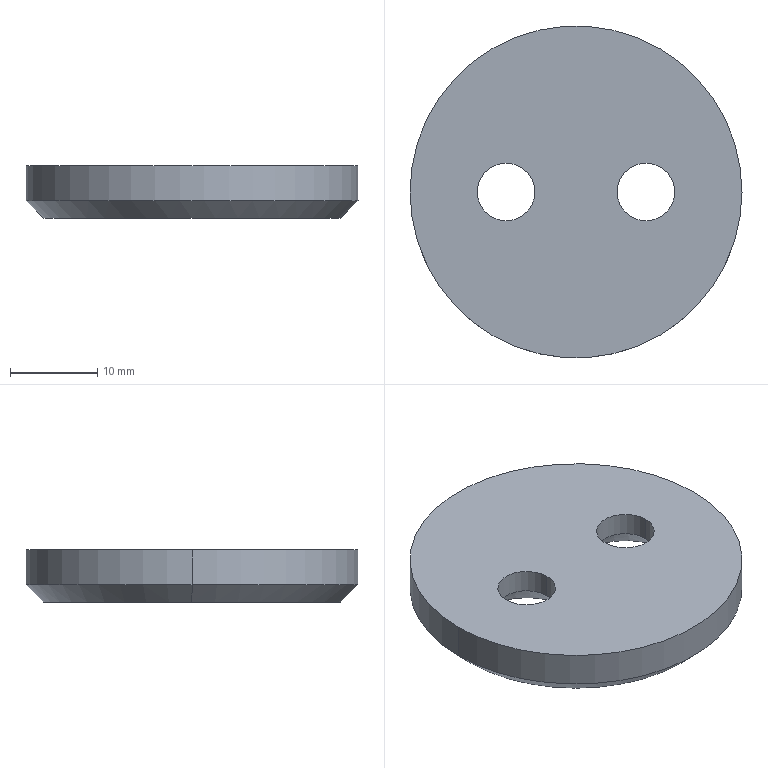Part | SolidWorks | features BaseBody 1 | 1 solid | 14 faces | box 38 x 38 x 6 mm | volume 5863 mm3 | cone 6 | cylinder 6 | plane 2 | commonest cylinder face diameters 6.6 x4 38 x2
STEP:
#1=CARTESIAN_POINT('',(11.3,0.,0.3));
#2=VERTEX_POINT('',#1);
#3=CARTESIAN_POINT('',(4.7,0.,0.3));
#4=VERTEX_POINT('',#3);
#5=CARTESIAN_POINT('',(8.,0.,0.3));
#6=DIRECTION('',(0.,0.,-1.));
#7=DIRECTION('',(-1.,0.,0.));
#8=AXIS2_PLACEMENT_3D('',#5,#6,#7);
#9=CIRCLE('',#8,3.3);
#10=EDGE_CURVE('',#2,#4,#9,.T.);
#11=ORIENTED_EDGE('',*,*,#10,.F.);
#12=CARTESIAN_POINT('',(14.6,0.,-3.));
#13=VERTEX_POINT('',#12);
#14=CARTESIAN_POINT('',(14.6,0.,-3.));
#15=DIRECTION('',(0.7071,0.,-0.7071));
#16=VECTOR('',#15,1000.);
#17=LINE('',#14,#16);
#18=EDGE_CURVE('',#2,#13,#17,.T.);
#19=ORIENTED_EDGE('',*,*,#18,.T.);
#20=CARTESIAN_POINT('',(1.4,0.,-3.));
#21=VERTEX_POINT('',#20);
#22=CARTESIAN_POINT('',(8.,0.,-3.));
#23=DIRECTION('',(0.,0.,-1.));
#24=DIRECTION('',(-1.,0.,0.));
#25=AXIS2_PLACEMENT_3D('',#22,#23,#24);
#26=CIRCLE('',#25,6.6);
#27=EDGE_CURVE('',#13,#21,#26,.T.);
#28=ORIENTED_EDGE('',*,*,#27,.T.);
#29=CARTESIAN_POINT('',(1.4,0.,-3.));
#30=DIRECTION('',(-0.7071,0.,-0.7071));
#31=VECTOR('',#30,1000.);
#32=LINE('',#29,#31);
#33=EDGE_CURVE('',#4,#21,#32,.T.);
#34=ORIENTED_EDGE('',*,*,#33,.F.);
#35=EDGE_LOOP('',(#11,#19,#28,#34));
#36=FACE_OUTER_BOUND('',#35,.T.);
#37=CARTESIAN_POINT('',(8.,0.,-3.));
#38=DIRECTION('',(0.,0.,-1.));
#39=DIRECTION('',(-1.,0.,0.));
#40=AXIS2_PLACEMENT_3D('',#37,#38,#39);
#41=CONICAL_SURFACE('',#40,6.6,0.7854);
#42=ADVANCED_FACE('',(#36),#41,.F.);
#43=CARTESIAN_POINT('',(11.3,0.,3.));
#44=VERTEX_POINT('',#43);
#45=CARTESIAN_POINT('',(4.7,0.,3.));
#46=VERTEX_POINT('',#45);
#47=CARTESIAN_POINT('',(8.,0.,3.));
#48=DIRECTION('',(0.,0.,-1.));
#49=DIRECTION('',(-1.,0.,0.));
#50=AXIS2_PLACEMENT_3D('',#47,#48,#49);
#51=CIRCLE('',#50,3.3);
#52=EDGE_CURVE('',#44,#46,#51,.T.);
#53=ORIENTED_EDGE('',*,*,#52,.F.);
#54=CARTESIAN_POINT('',(11.3,0.,-3.));
#55=DIRECTION('',(0.,0.,-1.));
#56=VECTOR('',#55,1000.);
#57=LINE('',#54,#56);
#58=EDGE_CURVE('',#44,#2,#57,.T.);
#59=ORIENTED_EDGE('',*,*,#58,.T.);
#60=ORIENTED_EDGE('',*,*,#10,.T.);
#61=CARTESIAN_POINT('',(4.7,0.,-3.));
#62=DIRECTION('',(0.,0.,-1.));
#63=VECTOR('',#62,1000.);
#64=LINE('',#61,#63);
#65=EDGE_CURVE('',#46,#4,#64,.T.);
#66=ORIENTED_EDGE('',*,*,#65,.F.);
#67=EDGE_LOOP('',(#53,#59,#60,#66));
#68=FACE_OUTER_BOUND('',#67,.T.);
#69=CARTESIAN_POINT('',(8.,0.,-3.));
#70=DIRECTION('',(0.,0.,-1.));
#71=DIRECTION('',(-1.,0.,0.));
#72=AXIS2_PLACEMENT_3D('',#69,#70,#71);
#73=CYLINDRICAL_SURFACE('',#72,3.3);
#74=ADVANCED_FACE('',(#68),#73,.F.);
#75=CARTESIAN_POINT('',(-4.7,0.,0.3));
#76=VERTEX_POINT('',#75);
#77=CARTESIAN_POINT('',(-11.3,0.,0.3));
#78=VERTEX_POINT('',#77);
#79=CARTESIAN_POINT('',(-8.,0.,0.3));
#80=DIRECTION('',(0.,0.,-1.));
#81=DIRECTION('',(-1.,0.,0.));
#82=AXIS2_PLACEMENT_3D('',#79,#80,#81);
#83=CIRCLE('',#82,3.3);
#84=EDGE_CURVE('',#76,#78,#83,.T.);
#85=ORIENTED_EDGE('',*,*,#84,.F.);
#86=CARTESIAN_POINT('',(-1.4,0.,-3.));
#87=VERTEX_POINT('',#86);
#88=CARTESIAN_POINT('',(-1.4,0.,-3.));
#89=DIRECTION('',(0.7071,0.,-0.7071));
#90=VECTOR('',#89,1000.);
#91=LINE('',#88,#90);
#92=EDGE_CURVE('',#76,#87,#91,.T.);
#93=ORIENTED_EDGE('',*,*,#92,.T.);
#94=CARTESIAN_POINT('',(-14.6,0.,-3.));
#95=VERTEX_POINT('',#94);
#96=CARTESIAN_POINT('',(-8.,0.,-3.));
#97=DIRECTION('',(0.,0.,-1.));
#98=DIRECTION('',(-1.,0.,0.));
#99=AXIS2_PLACEMENT_3D('',#96,#97,#98);
#100=CIRCLE('',#99,6.6);
#101=EDGE_CURVE('',#87,#95,#100,.T.);
#102=ORIENTED_EDGE('',*,*,#101,.T.);
#103=CARTESIAN_POINT('',(-14.6,0.,-3.));
#104=DIRECTION('',(-0.7071,0.,-0.7071));
#105=VECTOR('',#104,1000.);
#106=LINE('',#103,#105);
#107=EDGE_CURVE('',#78,#95,#106,.T.);
#108=ORIENTED_EDGE('',*,*,#107,.F.);
#109=EDGE_LOOP('',(#85,#93,#102,#108));
#110=FACE_OUTER_BOUND('',#109,.T.);
#111=CARTESIAN_POINT('',(-8.,0.,-3.));
#112=DIRECTION('',(0.,0.,-1.));
#113=DIRECTION('',(-1.,0.,0.));
#114=AXIS2_PLACEMENT_3D('',#111,#112,#113);
#115=CONICAL_SURFACE('',#114,6.6,0.7854);
#116=ADVANCED_FACE('',(#110),#115,.F.);
#117=CARTESIAN_POINT('',(-4.7,0.,3.));
#118=VERTEX_POINT('',#117);
#119=CARTESIAN_POINT('',(-11.3,0.,3.));
#120=VERTEX_POINT('',#119);
#121=CARTESIAN_POINT('',(-8.,0.,3.));
#122=DIRECTION('',(0.,0.,-1.));
#123=DIRECTION('',(-1.,0.,0.));
#124=AXIS2_PLACEMENT_3D('',#121,#122,#123);
#125=CIRCLE('',#124,3.3);
#126=EDGE_CURVE('',#118,#120,#125,.T.);
#127=ORIENTED_EDGE('',*,*,#126,.F.);
#128=CARTESIAN_POINT('',(-4.7,0.,-3.));
#129=DIRECTION('',(0.,0.,-1.));
#130=VECTOR('',#129,1000.);
#131=LINE('',#128,#130);
#132=EDGE_CURVE('',#118,#76,#131,.T.);
#133=ORIENTED_EDGE('',*,*,#132,.T.);
#134=ORIENTED_EDGE('',*,*,#84,.T.);
#135=CARTESIAN_POINT('',(-11.3,0.,-3.));
#136=DIRECTION('',(0.,0.,-1.));
#137=VECTOR('',#136,1000.);
#138=LINE('',#135,#137);
#139=EDGE_CURVE('',#120,#78,#138,.T.);
#140=ORIENTED_EDGE('',*,*,#139,.F.);
#141=EDGE_LOOP('',(#127,#133,#134,#140));
#142=FACE_OUTER_BOUND('',#141,.T.);
#143=CARTESIAN_POINT('',(-8.,0.,-3.));
#144=DIRECTION('',(0.,0.,-1.));
#145=DIRECTION('',(-1.,0.,0.));
#146=AXIS2_PLACEMENT_3D('',#143,#144,#145);
#147=CYLINDRICAL_SURFACE('',#146,3.3);
#148=ADVANCED_FACE('',(#142),#147,.F.);
#149=CARTESIAN_POINT('',(-17.,0.,-3.));
#150=VERTEX_POINT('',#149);
#151=CARTESIAN_POINT('',(17.,0.,-3.));
#152=VERTEX_POINT('',#151);
#153=CARTESIAN_POINT('',(0.,0.,-3.));
#154=DIRECTION('',(0.,0.,-1.));
#155=DIRECTION('',(1.,0.,0.));
#156=AXIS2_PLACEMENT_3D('',#153,#154,#155);
#157=CIRCLE('',#156,17.);
#158=EDGE_CURVE('',#150,#152,#157,.T.);
#159=ORIENTED_EDGE('',*,*,#158,.F.);
#160=CARTESIAN_POINT('',(-19.,0.,-1.));
#161=VERTEX_POINT('',#160);
#162=CARTESIAN_POINT('',(-19.,0.,-1.));
#163=DIRECTION('',(-0.7071,0.,0.7071));
#164=VECTOR('',#163,1000.);
#165=LINE('',#162,#164);
#166=EDGE_CURVE('',#150,#161,#165,.T.);
#167=ORIENTED_EDGE('',*,*,#166,.T.);
#168=CARTESIAN_POINT('',(19.,0.,-1.));
#169=VERTEX_POINT('',#168);
#170=CARTESIAN_POINT('',(0.,0.,-1.));
#171=DIRECTION('',(0.,0.,1.));
#172=DIRECTION('',(1.,0.,0.));
#173=AXIS2_PLACEMENT_3D('',#170,#171,#172);
#174=CIRCLE('',#173,19.);
#175=EDGE_CURVE('',#169,#161,#174,.T.);
#176=ORIENTED_EDGE('',*,*,#175,.F.);
#177=CARTESIAN_POINT('',(19.,0.,-1.));
#178=DIRECTION('',(0.7071,0.,0.7071));
#179=VECTOR('',#178,1000.);
#180=LINE('',#177,#179);
#181=EDGE_CURVE('',#152,#169,#180,.T.);
#182=ORIENTED_EDGE('',*,*,#181,.F.);
#183=EDGE_LOOP('',(#159,#167,#176,#182));
#184=FACE_OUTER_BOUND('',#183,.T.);
#185=CARTESIAN_POINT('',(0.,0.,-1.));
#186=DIRECTION('',(0.,0.,1.));
#187=DIRECTION('',(1.,0.,0.));
#188=AXIS2_PLACEMENT_3D('',#185,#186,#187);
#189=CONICAL_SURFACE('',#188,19.,0.7854);
#190=ADVANCED_FACE('',(#184),#189,.T.);
#191=CARTESIAN_POINT('',(19.,0.,3.));
#192=VERTEX_POINT('',#191);
#193=CARTESIAN_POINT('',(-19.,0.,3.));
#194=VERTEX_POINT('',#193);
#195=CARTESIAN_POINT('',(0.,0.,3.));
#196=DIRECTION('',(0.,0.,1.));
#197=DIRECTION('',(1.,0.,0.));
#198=AXIS2_PLACEMENT_3D('',#195,#196,#197);
#199=CIRCLE('',#198,19.);
#200=EDGE_CURVE('',#192,#194,#199,.T.);
#201=ORIENTED_EDGE('',*,*,#200,.F.);
#202=CARTESIAN_POINT('',(19.,0.,3.));
#203=DIRECTION('',(0.,0.,-1.));
#204=VECTOR('',#203,1000.);
#205=LINE('',#202,#204);
#206=EDGE_CURVE('',#192,#169,#205,.T.);
#207=ORIENTED_EDGE('',*,*,#206,.T.);
#208=ORIENTED_EDGE('',*,*,#175,.T.);
#209=CARTESIAN_POINT('',(-19.,0.,3.));
#210=DIRECTION('',(0.,0.,-1.));
#211=VECTOR('',#210,1000.);
#212=LINE('',#209,#211);
#213=EDGE_CURVE('',#194,#161,#212,.T.);
#214=ORIENTED_EDGE('',*,*,#213,.F.);
#215=EDGE_LOOP('',(#201,#207,#208,#214));
#216=FACE_OUTER_BOUND('',#215,.T.);
#217=CARTESIAN_POINT('',(0.,0.,3.));
#218=DIRECTION('',(0.,0.,-1.));
#219=DIRECTION('',(-1.,0.,0.));
#220=AXIS2_PLACEMENT_3D('',#217,#218,#219);
#221=CYLINDRICAL_SURFACE('',#220,19.);
#222=ADVANCED_FACE('',(#216),#221,.T.);
#223=CARTESIAN_POINT('',(-8.,0.,-3.));
#224=DIRECTION('',(0.,0.,-1.));
#225=DIRECTION('',(-1.,0.,0.));
#226=AXIS2_PLACEMENT_3D('',#223,#224,#225);
#227=CIRCLE('',#226,6.6);
#228=EDGE_CURVE('',#95,#87,#227,.T.);
#229=ORIENTED_EDGE('',*,*,#228,.F.);
#230=ORIENTED_EDGE('',*,*,#101,.F.);
#231=EDGE_LOOP('',(#229,#230));
#232=FACE_BOUND('',#231,.T.);
#233=CARTESIAN_POINT('',(8.,0.,-3.));
#234=DIRECTION('',(0.,0.,-1.));
#235=DIRECTION('',(-1.,0.,0.));
#236=AXIS2_PLACEMENT_3D('',#233,#234,#235);
#237=CIRCLE('',#236,6.6);
#238=EDGE_CURVE('',#21,#13,#237,.T.);
#239=ORIENTED_EDGE('',*,*,#238,.F.);
#240=ORIENTED_EDGE('',*,*,#27,.F.);
#241=EDGE_LOOP('',(#239,#240));
#242=FACE_BOUND('',#241,.T.);
#243=CARTESIAN_POINT('',(0.,0.,-3.));
#244=DIRECTION('',(0.,0.,-1.));
#245=DIRECTION('',(1.,0.,0.));
#246=AXIS2_PLACEMENT_3D('',#243,#244,#245);
#247=CIRCLE('',#246,17.);
#248=EDGE_CURVE('',#152,#150,#247,.T.);
#249=ORIENTED_EDGE('',*,*,#248,.T.);
#250=ORIENTED_EDGE('',*,*,#158,.T.);
#251=EDGE_LOOP('',(#249,#250));
#252=FACE_OUTER_BOUND('',#251,.T.);
#253=CARTESIAN_POINT('',(0.,0.,-3.));
#254=DIRECTION('',(0.,0.,1.));
#255=DIRECTION('',(0.,-1.,0.));
#256=AXIS2_PLACEMENT_3D('',#253,#254,#255);
#257=PLANE('',#256);
#258=ADVANCED_FACE('',(#232,#242,#252),#257,.F.);
#259=CARTESIAN_POINT('',(-8.,0.,3.));
#260=DIRECTION('',(0.,0.,-1.));
#261=DIRECTION('',(-1.,0.,0.));
#262=AXIS2_PLACEMENT_3D('',#259,#260,#261);
#263=CIRCLE('',#262,3.3);
#264=EDGE_CURVE('',#120,#118,#263,.T.);
#265=ORIENTED_EDGE('',*,*,#264,.T.);
#266=ORIENTED_EDGE('',*,*,#126,.T.);
#267=EDGE_LOOP('',(#265,#266));
#268=FACE_BOUND('',#267,.T.);
#269=CARTESIAN_POINT('',(8.,0.,3.));
#270=DIRECTION('',(0.,0.,-1.));
#271=DIRECTION('',(-1.,0.,0.));
#272=AXIS2_PLACEMENT_3D('',#269,#270,#271);
#273=CIRCLE('',#272,3.3);
#274=EDGE_CURVE('',#46,#44,#273,.T.);
#275=ORIENTED_EDGE('',*,*,#274,.T.);
#276=ORIENTED_EDGE('',*,*,#52,.T.);
#277=EDGE_LOOP('',(#275,#276));
#278=FACE_BOUND('',#277,.T.);
#279=CARTESIAN_POINT('',(0.,0.,3.));
#280=DIRECTION('',(0.,0.,1.));
#281=DIRECTION('',(1.,0.,0.));
#282=AXIS2_PLACEMENT_3D('',#279,#280,#281);
#283=CIRCLE('',#282,19.);
#284=EDGE_CURVE('',#194,#192,#283,.T.);
#285=ORIENTED_EDGE('',*,*,#284,.T.);
#286=ORIENTED_EDGE('',*,*,#200,.T.);
#287=EDGE_LOOP('',(#285,#286));
#288=FACE_OUTER_BOUND('',#287,.T.);
#289=CARTESIAN_POINT('',(0.,0.,3.));
#290=DIRECTION('',(0.,0.,1.));
#291=DIRECTION('',(0.,-1.,0.));
#292=AXIS2_PLACEMENT_3D('',#289,#290,#291);
#293=PLANE('',#292);
#294=ADVANCED_FACE('',(#268,#278,#288),#293,.T.);
#295=ORIENTED_EDGE('',*,*,#206,.F.);
#296=ORIENTED_EDGE('',*,*,#284,.F.);
#297=ORIENTED_EDGE('',*,*,#213,.T.);
#298=CARTESIAN_POINT('',(0.,0.,-1.));
#299=DIRECTION('',(0.,0.,1.));
#300=DIRECTION('',(1.,0.,0.));
#301=AXIS2_PLACEMENT_3D('',#298,#299,#300);
#302=CIRCLE('',#301,19.);
#303=EDGE_CURVE('',#161,#169,#302,.T.);
#304=ORIENTED_EDGE('',*,*,#303,.T.);
#305=EDGE_LOOP('',(#295,#296,#297,#304));
#306=FACE_OUTER_BOUND('',#305,.T.);
#307=CARTESIAN_POINT('',(0.,0.,3.));
#308=DIRECTION('',(0.,0.,-1.));
#309=DIRECTION('',(-1.,0.,0.));
#310=AXIS2_PLACEMENT_3D('',#307,#308,#309);
#311=CYLINDRICAL_SURFACE('',#310,19.);
#312=ADVANCED_FACE('',(#306),#311,.T.);
#313=ORIENTED_EDGE('',*,*,#166,.F.);
#314=ORIENTED_EDGE('',*,*,#248,.F.);
#315=ORIENTED_EDGE('',*,*,#181,.T.);
#316=ORIENTED_EDGE('',*,*,#303,.F.);
#317=EDGE_LOOP('',(#313,#314,#315,#316));
#318=FACE_OUTER_BOUND('',#317,.T.);
#319=CARTESIAN_POINT('',(0.,0.,-1.));
#320=DIRECTION('',(0.,0.,1.));
#321=DIRECTION('',(1.,0.,0.));
#322=AXIS2_PLACEMENT_3D('',#319,#320,#321);
#323=CONICAL_SURFACE('',#322,19.,0.7854);
#324=ADVANCED_FACE('',(#318),#323,.T.);
#325=ORIENTED_EDGE('',*,*,#132,.F.);
#326=ORIENTED_EDGE('',*,*,#264,.F.);
#327=ORIENTED_EDGE('',*,*,#139,.T.);
#328=CARTESIAN_POINT('',(-8.,0.,0.3));
#329=DIRECTION('',(0.,0.,-1.));
#330=DIRECTION('',(-1.,0.,0.));
#331=AXIS2_PLACEMENT_3D('',#328,#329,#330);
#332=CIRCLE('',#331,3.3);
#333=EDGE_CURVE('',#78,#76,#332,.T.);
#334=ORIENTED_EDGE('',*,*,#333,.T.);
#335=EDGE_LOOP('',(#325,#326,#327,#334));
#336=FACE_OUTER_BOUND('',#335,.T.);
#337=CARTESIAN_POINT('',(-8.,0.,-3.));
#338=DIRECTION('',(0.,0.,-1.));
#339=DIRECTION('',(-1.,0.,0.));
#340=AXIS2_PLACEMENT_3D('',#337,#338,#339);
#341=CYLINDRICAL_SURFACE('',#340,3.3);
#342=ADVANCED_FACE('',(#336),#341,.F.);
#343=ORIENTED_EDGE('',*,*,#92,.F.);
#344=ORIENTED_EDGE('',*,*,#333,.F.);
#345=ORIENTED_EDGE('',*,*,#107,.T.);
#346=ORIENTED_EDGE('',*,*,#228,.T.);
#347=EDGE_LOOP('',(#343,#344,#345,#346));
#348=FACE_OUTER_BOUND('',#347,.T.);
#349=CARTESIAN_POINT('',(-8.,0.,-3.));
#350=DIRECTION('',(0.,0.,-1.));
#351=DIRECTION('',(-1.,0.,0.));
#352=AXIS2_PLACEMENT_3D('',#349,#350,#351);
#353=CONICAL_SURFACE('',#352,6.6,0.7854);
#354=ADVANCED_FACE('',(#348),#353,.F.);
#355=ORIENTED_EDGE('',*,*,#58,.F.);
#356=ORIENTED_EDGE('',*,*,#274,.F.);
#357=ORIENTED_EDGE('',*,*,#65,.T.);
#358=CARTESIAN_POINT('',(8.,0.,0.3));
#359=DIRECTION('',(0.,0.,-1.));
#360=DIRECTION('',(-1.,0.,0.));
#361=AXIS2_PLACEMENT_3D('',#358,#359,#360);
#362=CIRCLE('',#361,3.3);
#363=EDGE_CURVE('',#4,#2,#362,.T.);
#364=ORIENTED_EDGE('',*,*,#363,.T.);
#365=EDGE_LOOP('',(#355,#356,#357,#364));
#366=FACE_OUTER_BOUND('',#365,.T.);
#367=CARTESIAN_POINT('',(8.,0.,-3.));
#368=DIRECTION('',(0.,0.,-1.));
#369=DIRECTION('',(-1.,0.,0.));
#370=AXIS2_PLACEMENT_3D('',#367,#368,#369);
#371=CYLINDRICAL_SURFACE('',#370,3.3);
#372=ADVANCED_FACE('',(#366),#371,.F.);
#373=ORIENTED_EDGE('',*,*,#18,.F.);
#374=ORIENTED_EDGE('',*,*,#363,.F.);
#375=ORIENTED_EDGE('',*,*,#33,.T.);
#376=ORIENTED_EDGE('',*,*,#238,.T.);
#377=EDGE_LOOP('',(#373,#374,#375,#376));
#378=FACE_OUTER_BOUND('',#377,.T.);
#379=CARTESIAN_POINT('',(8.,0.,-3.));
#380=DIRECTION('',(0.,0.,-1.));
#381=DIRECTION('',(-1.,0.,0.));
#382=AXIS2_PLACEMENT_3D('',#379,#380,#381);
#383=CONICAL_SURFACE('',#382,6.6,0.7854);
#384=ADVANCED_FACE('',(#378),#383,.F.);
#385=CLOSED_SHELL('',(#42,#74,#116,#148,#190,#222,#258,#294,#312,#324,#342,#354,#372,#384));
#386=MANIFOLD_SOLID_BREP('',#385);
#387=CARTESIAN_POINT('',(0.,0.,0.));
#388=DIRECTION('',(0.,0.,1.));
#389=DIRECTION('',(1.,0.,0.));
#390=AXIS2_PLACEMENT_3D('',#387,#388,#389);
#391=(LENGTH_UNIT()NAMED_UNIT(*)SI_UNIT(.MILLI.,.METRE.));
#392=UNCERTAINTY_MEASURE_WITH_UNIT(LENGTH_MEASURE(0.00001),#391,'','');
#393=(NAMED_UNIT(*)PLANE_ANGLE_UNIT()SI_UNIT($,.RADIAN.));
#394=(NAMED_UNIT(*)SI_UNIT($,.STERADIAN.)SOLID_ANGLE_UNIT());
#395=(GEOMETRIC_REPRESENTATION_CONTEXT(3)GLOBAL_UNCERTAINTY_ASSIGNED_CONTEXT((#392))GLOBAL_UNIT_ASSIGNED_CONTEXT((#391,#393,#394))REPRESENTATION_CONTEXT('',''));
#396=ADVANCED_BREP_SHAPE_REPRESENTATION('',(#386,#390),#395);